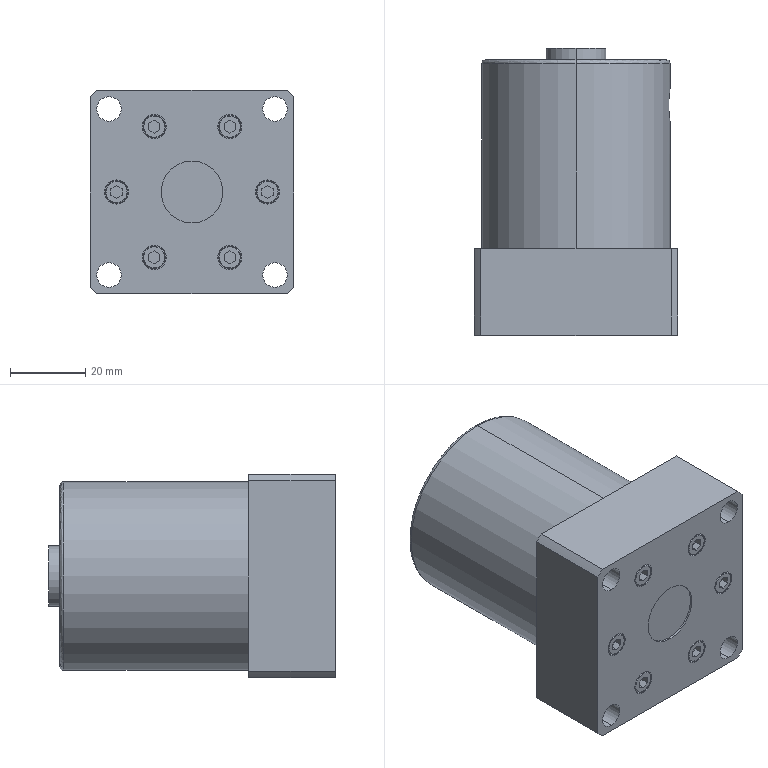Part | STEP file | rotary cylinder ACKL32x90 | 2 solids | 161 faces | box 54 x 76 x 54 mm | volume 144312 mm3 | plane 67 | cylinder 62 | cone 18 | spline 14 | commonest cylinder face diameters 6 x12 6.4 x12 2 x8 6.5 x8 8.566 x4 16 x4